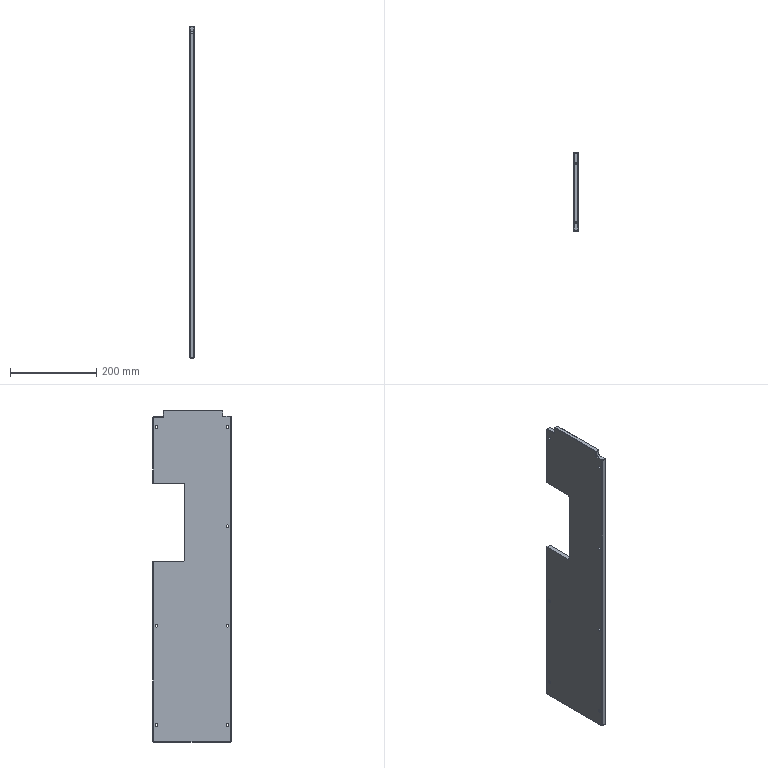Part | NX | 1 solid | 65 faces | box 10 x 182 x 768 mm | volume 1252221 mm3 | plane 32 | cylinder 17 | cone 16 | commonest cylinder face diameters 4 x8 6.5 x7 10 x2